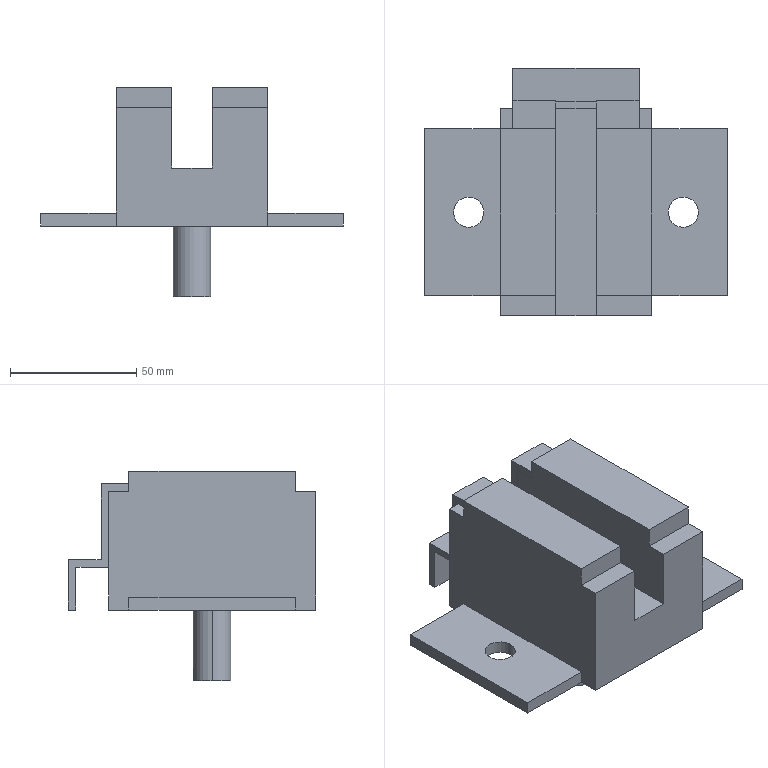Part | 2 solids | 51 faces | box 120 x 98 x 83 mm | volume 255571 mm3 | plane 45 | cylinder 6 | commonest cylinder face diameters 12 x4 15 x2
STEP:
#1=CARTESIAN_POINT('',(-48.5,0.,0.));
#2=VERTEX_POINT('',#1);
#3=CARTESIAN_POINT('',(-36.5,0.,0.));
#4=VERTEX_POINT('',#3);
#5=CARTESIAN_POINT('',(-42.5,0.,0.));
#6=DIRECTION('',(0.,0.,1.));
#7=DIRECTION('',(1.,0.,0.));
#8=AXIS2_PLACEMENT_3D('',#5,#6,#7);
#9=CIRCLE('',#8,6.);
#10=EDGE_CURVE('',#2,#4,#9,.T.);
#11=ORIENTED_EDGE('',*,*,#10,.F.);
#12=CARTESIAN_POINT('',(-48.5,0.,5.));
#13=VERTEX_POINT('',#12);
#14=CARTESIAN_POINT('',(-48.5,0.,-23.));
#15=DIRECTION('',(0.,0.,1.));
#16=VECTOR('',#15,1000.);
#17=LINE('',#14,#16);
#18=EDGE_CURVE('',#2,#13,#17,.T.);
#19=ORIENTED_EDGE('',*,*,#18,.T.);
#20=CARTESIAN_POINT('',(-36.5,0.,5.));
#21=VERTEX_POINT('',#20);
#22=CARTESIAN_POINT('',(-42.5,0.,5.));
#23=DIRECTION('',(0.,0.,1.));
#24=DIRECTION('',(1.,0.,0.));
#25=AXIS2_PLACEMENT_3D('',#22,#23,#24);
#26=CIRCLE('',#25,6.);
#27=EDGE_CURVE('',#13,#21,#26,.T.);
#28=ORIENTED_EDGE('',*,*,#27,.T.);
#29=CARTESIAN_POINT('',(-36.5,0.,-23.));
#30=DIRECTION('',(0.,0.,1.));
#31=VECTOR('',#30,1000.);
#32=LINE('',#29,#31);
#33=EDGE_CURVE('',#4,#21,#32,.T.);
#34=ORIENTED_EDGE('',*,*,#33,.F.);
#35=EDGE_LOOP('',(#11,#19,#28,#34));
#36=FACE_OUTER_BOUND('',#35,.T.);
#37=CARTESIAN_POINT('',(-42.5,0.,-23.));
#38=DIRECTION('',(0.,0.,1.));
#39=DIRECTION('',(1.,0.,0.));
#40=AXIS2_PLACEMENT_3D('',#37,#38,#39);
#41=CYLINDRICAL_SURFACE('',#40,6.);
#42=ADVANCED_FACE('',(#36),#41,.F.);
#43=CARTESIAN_POINT('',(36.5,0.,0.));
#44=VERTEX_POINT('',#43);
#45=CARTESIAN_POINT('',(48.5,0.,0.));
#46=VERTEX_POINT('',#45);
#47=CARTESIAN_POINT('',(42.5,0.,0.));
#48=DIRECTION('',(0.,0.,1.));
#49=DIRECTION('',(1.,0.,0.));
#50=AXIS2_PLACEMENT_3D('',#47,#48,#49);
#51=CIRCLE('',#50,6.);
#52=EDGE_CURVE('',#44,#46,#51,.T.);
#53=ORIENTED_EDGE('',*,*,#52,.F.);
#54=CARTESIAN_POINT('',(36.5,0.,5.));
#55=VERTEX_POINT('',#54);
#56=CARTESIAN_POINT('',(36.5,0.,-23.));
#57=DIRECTION('',(0.,0.,1.));
#58=VECTOR('',#57,1000.);
#59=LINE('',#56,#58);
#60=EDGE_CURVE('',#44,#55,#59,.T.);
#61=ORIENTED_EDGE('',*,*,#60,.T.);
#62=CARTESIAN_POINT('',(48.5,0.,5.));
#63=VERTEX_POINT('',#62);
#64=CARTESIAN_POINT('',(42.5,0.,5.));
#65=DIRECTION('',(0.,0.,1.));
#66=DIRECTION('',(-1.,0.,0.));
#67=AXIS2_PLACEMENT_3D('',#64,#65,#66);
#68=CIRCLE('',#67,6.);
#69=EDGE_CURVE('',#55,#63,#68,.T.);
#70=ORIENTED_EDGE('',*,*,#69,.T.);
#71=CARTESIAN_POINT('',(48.5,0.,-23.));
#72=DIRECTION('',(0.,0.,1.));
#73=VECTOR('',#72,1000.);
#74=LINE('',#71,#73);
#75=EDGE_CURVE('',#46,#63,#74,.T.);
#76=ORIENTED_EDGE('',*,*,#75,.F.);
#77=EDGE_LOOP('',(#53,#61,#70,#76));
#78=FACE_OUTER_BOUND('',#77,.T.);
#79=CARTESIAN_POINT('',(42.5,0.,-23.));
#80=DIRECTION('',(0.,0.,1.));
#81=DIRECTION('',(1.,0.,0.));
#82=AXIS2_PLACEMENT_3D('',#79,#80,#81);
#83=CYLINDRICAL_SURFACE('',#82,6.);
#84=ADVANCED_FACE('',(#78),#83,.F.);
#85=CARTESIAN_POINT('',(-7.5,0.,-28.));
#86=VERTEX_POINT('',#85);
#87=CARTESIAN_POINT('',(7.5,0.,-28.));
#88=VERTEX_POINT('',#87);
#89=CARTESIAN_POINT('',(0.,0.,-28.));
#90=DIRECTION('',(0.,0.,-1.));
#91=DIRECTION('',(-1.,0.,0.));
#92=AXIS2_PLACEMENT_3D('',#89,#90,#91);
#93=CIRCLE('',#92,7.5);
#94=EDGE_CURVE('',#86,#88,#93,.T.);
#95=ORIENTED_EDGE('',*,*,#94,.F.);
#96=CARTESIAN_POINT('',(-7.5,0.,0.));
#97=VERTEX_POINT('',#96);
#98=CARTESIAN_POINT('',(-7.5,0.,-28.));
#99=DIRECTION('',(0.,0.,1.));
#100=VECTOR('',#99,1000.);
#101=LINE('',#98,#100);
#102=EDGE_CURVE('',#86,#97,#101,.T.);
#103=ORIENTED_EDGE('',*,*,#102,.T.);
#104=CARTESIAN_POINT('',(7.5,0.,0.));
#105=VERTEX_POINT('',#104);
#106=CARTESIAN_POINT('',(0.,0.,0.));
#107=DIRECTION('',(0.,0.,-1.));
#108=DIRECTION('',(1.,0.,0.));
#109=AXIS2_PLACEMENT_3D('',#106,#107,#108);
#110=CIRCLE('',#109,7.5);
#111=EDGE_CURVE('',#97,#105,#110,.T.);
#112=ORIENTED_EDGE('',*,*,#111,.T.);
#113=CARTESIAN_POINT('',(7.5,0.,-28.));
#114=DIRECTION('',(0.,0.,1.));
#115=VECTOR('',#114,1000.);
#116=LINE('',#113,#115);
#117=EDGE_CURVE('',#88,#105,#116,.T.);
#118=ORIENTED_EDGE('',*,*,#117,.F.);
#119=EDGE_LOOP('',(#95,#103,#112,#118));
#120=FACE_OUTER_BOUND('',#119,.T.);
#121=CARTESIAN_POINT('',(0.,0.,-28.));
#122=DIRECTION('',(0.,0.,1.));
#123=DIRECTION('',(1.,0.,0.));
#124=AXIS2_PLACEMENT_3D('',#121,#122,#123);
#125=CYLINDRICAL_SURFACE('',#124,7.5);
#126=ADVANCED_FACE('',(#120),#125,.T.);
#127=CARTESIAN_POINT('',(30.,-33.,5.));
#128=VERTEX_POINT('',#127);
#129=CARTESIAN_POINT('',(60.,-33.,5.));
#130=VERTEX_POINT('',#129);
#131=CARTESIAN_POINT('',(-60.,-33.,5.));
#132=DIRECTION('',(1.,0.,0.));
#133=VECTOR('',#132,1000.);
#134=LINE('',#131,#133);
#135=EDGE_CURVE('',#128,#130,#134,.T.);
#136=ORIENTED_EDGE('',*,*,#135,.F.);
#137=CARTESIAN_POINT('',(30.,-33.,0.));
#138=VERTEX_POINT('',#137);
#139=CARTESIAN_POINT('',(30.,-33.,55.));
#140=DIRECTION('',(0.,0.,-1.));
#141=VECTOR('',#140,1000.);
#142=LINE('',#139,#141);
#143=EDGE_CURVE('',#128,#138,#142,.T.);
#144=ORIENTED_EDGE('',*,*,#143,.T.);
#145=CARTESIAN_POINT('',(60.,-33.,0.));
#146=VERTEX_POINT('',#145);
#147=CARTESIAN_POINT('',(-60.,-33.,0.));
#148=DIRECTION('',(1.,0.,0.));
#149=VECTOR('',#148,1000.);
#150=LINE('',#147,#149);
#151=EDGE_CURVE('',#138,#146,#150,.T.);
#152=ORIENTED_EDGE('',*,*,#151,.T.);
#153=CARTESIAN_POINT('',(60.,-33.,5.));
#154=DIRECTION('',(0.,0.,-1.));
#155=VECTOR('',#154,1000.);
#156=LINE('',#153,#155);
#157=EDGE_CURVE('',#130,#146,#156,.T.);
#158=ORIENTED_EDGE('',*,*,#157,.F.);
#159=EDGE_LOOP('',(#136,#144,#152,#158));
#160=FACE_OUTER_BOUND('',#159,.T.);
#161=CARTESIAN_POINT('',(-60.,-33.,5.));
#162=DIRECTION('',(0.,1.,0.));
#163=DIRECTION('',(0.,0.,1.));
#164=AXIS2_PLACEMENT_3D('',#161,#162,#163);
#165=PLANE('',#164);
#166=ADVANCED_FACE('',(#160),#165,.F.);
#167=CARTESIAN_POINT('',(-30.,33.,0.));
#168=VERTEX_POINT('',#167);
#169=CARTESIAN_POINT('',(-30.,33.,5.));
#170=VERTEX_POINT('',#169);
#171=CARTESIAN_POINT('',(-30.,33.,5.));
#172=DIRECTION('',(0.,0.,1.));
#173=VECTOR('',#172,1000.);
#174=LINE('',#171,#173);
#175=EDGE_CURVE('',#168,#170,#174,.T.);
#176=ORIENTED_EDGE('',*,*,#175,.F.);
#177=CARTESIAN_POINT('',(-60.,33.,0.));
#178=VERTEX_POINT('',#177);
#179=CARTESIAN_POINT('',(-60.,33.,0.));
#180=DIRECTION('',(-1.,0.,0.));
#181=VECTOR('',#180,1000.);
#182=LINE('',#179,#181);
#183=EDGE_CURVE('',#168,#178,#182,.T.);
#184=ORIENTED_EDGE('',*,*,#183,.T.);
#185=CARTESIAN_POINT('',(-60.,33.,5.));
#186=VERTEX_POINT('',#185);
#187=CARTESIAN_POINT('',(-60.,33.,5.));
#188=DIRECTION('',(0.,0.,-1.));
#189=VECTOR('',#188,1000.);
#190=LINE('',#187,#189);
#191=EDGE_CURVE('',#186,#178,#190,.T.);
#192=ORIENTED_EDGE('',*,*,#191,.F.);
#193=CARTESIAN_POINT('',(-60.,33.,5.));
#194=DIRECTION('',(-1.,0.,0.));
#195=VECTOR('',#194,1000.);
#196=LINE('',#193,#195);
#197=EDGE_CURVE('',#170,#186,#196,.T.);
#198=ORIENTED_EDGE('',*,*,#197,.F.);
#199=EDGE_LOOP('',(#176,#184,#192,#198));
#200=FACE_OUTER_BOUND('',#199,.T.);
#201=CARTESIAN_POINT('',(-60.,33.,5.));
#202=DIRECTION('',(0.,-1.,0.));
#203=DIRECTION('',(0.,0.,-1.));
#204=AXIS2_PLACEMENT_3D('',#201,#202,#203);
#205=PLANE('',#204);
#206=ADVANCED_FACE('',(#200),#205,.F.);
#207=CARTESIAN_POINT('',(30.,33.,5.));
#208=VERTEX_POINT('',#207);
#209=CARTESIAN_POINT('',(30.,33.,0.));
#210=VERTEX_POINT('',#209);
#211=CARTESIAN_POINT('',(30.,33.,5.));
#212=DIRECTION('',(0.,0.,-1.));
#213=VECTOR('',#212,1000.);
#214=LINE('',#211,#213);
#215=EDGE_CURVE('',#208,#210,#214,.T.);
#216=ORIENTED_EDGE('',*,*,#215,.F.);
#217=CARTESIAN_POINT('',(60.,33.,5.));
#218=VERTEX_POINT('',#217);
#219=CARTESIAN_POINT('',(-60.,33.,5.));
#220=DIRECTION('',(-1.,0.,0.));
#221=VECTOR('',#220,1000.);
#222=LINE('',#219,#221);
#223=EDGE_CURVE('',#218,#208,#222,.T.);
#224=ORIENTED_EDGE('',*,*,#223,.F.);
#225=CARTESIAN_POINT('',(60.,33.,0.));
#226=VERTEX_POINT('',#225);
#227=CARTESIAN_POINT('',(60.,33.,5.));
#228=DIRECTION('',(0.,0.,-1.));
#229=VECTOR('',#228,1000.);
#230=LINE('',#227,#229);
#231=EDGE_CURVE('',#218,#226,#230,.T.);
#232=ORIENTED_EDGE('',*,*,#231,.T.);
#233=CARTESIAN_POINT('',(-60.,33.,0.));
#234=DIRECTION('',(-1.,0.,0.));
#235=VECTOR('',#234,1000.);
#236=LINE('',#233,#235);
#237=EDGE_CURVE('',#226,#210,#236,.T.);
#238=ORIENTED_EDGE('',*,*,#237,.T.);
#239=EDGE_LOOP('',(#216,#224,#232,#238));
#240=FACE_OUTER_BOUND('',#239,.T.);
#241=CARTESIAN_POINT('',(-60.,33.,5.));
#242=DIRECTION('',(0.,-1.,0.));
#243=DIRECTION('',(0.,0.,-1.));
#244=AXIS2_PLACEMENT_3D('',#241,#242,#243);
#245=PLANE('',#244);
#246=ADVANCED_FACE('',(#240),#245,.F.);
#247=CARTESIAN_POINT('',(8.,33.,55.));
#248=VERTEX_POINT('',#247);
#249=CARTESIAN_POINT('',(30.,33.,55.));
#250=VERTEX_POINT('',#249);
#251=CARTESIAN_POINT('',(-60.,33.,55.));
#252=DIRECTION('',(1.,0.,0.));
#253=VECTOR('',#252,1000.);
#254=LINE('',#251,#253);
#255=EDGE_CURVE('',#248,#250,#254,.T.);
#256=ORIENTED_EDGE('',*,*,#255,.F.);
#257=CARTESIAN_POINT('',(8.,-33.,55.));
#258=VERTEX_POINT('',#257);
#259=CARTESIAN_POINT('',(8.,33.,55.));
#260=DIRECTION('',(0.,1.,0.));
#261=VECTOR('',#260,1000.);
#262=LINE('',#259,#261);
#263=EDGE_CURVE('',#258,#248,#262,.T.);
#264=ORIENTED_EDGE('',*,*,#263,.F.);
#265=CARTESIAN_POINT('',(30.,-33.,55.));
#266=VERTEX_POINT('',#265);
#267=CARTESIAN_POINT('',(-60.,-33.,55.));
#268=DIRECTION('',(1.,0.,0.));
#269=VECTOR('',#268,1000.);
#270=LINE('',#267,#269);
#271=EDGE_CURVE('',#258,#266,#270,.T.);
#272=ORIENTED_EDGE('',*,*,#271,.T.);
#273=CARTESIAN_POINT('',(30.,33.,55.));
#274=DIRECTION('',(0.,1.,0.));
#275=VECTOR('',#274,1000.);
#276=LINE('',#273,#275);
#277=EDGE_CURVE('',#266,#250,#276,.T.);
#278=ORIENTED_EDGE('',*,*,#277,.T.);
#279=EDGE_LOOP('',(#256,#264,#272,#278));
#280=FACE_OUTER_BOUND('',#279,.T.);
#281=CARTESIAN_POINT('',(0.,0.,55.));
#282=DIRECTION('',(0.,0.,1.));
#283=DIRECTION('',(1.,0.,0.));
#284=AXIS2_PLACEMENT_3D('',#281,#282,#283);
#285=PLANE('',#284);
#286=ADVANCED_FACE('',(#280),#285,.T.);
#287=CARTESIAN_POINT('',(42.5,0.,5.));
#288=DIRECTION('',(0.,0.,1.));
#289=DIRECTION('',(-1.,0.,0.));
#290=AXIS2_PLACEMENT_3D('',#287,#288,#289);
#291=CIRCLE('',#290,6.);
#292=EDGE_CURVE('',#63,#55,#291,.T.);
#293=ORIENTED_EDGE('',*,*,#292,.F.);
#294=ORIENTED_EDGE('',*,*,#69,.F.);
#295=EDGE_LOOP('',(#293,#294));
#296=FACE_BOUND('',#295,.T.);
#297=CARTESIAN_POINT('',(30.,33.,5.));
#298=DIRECTION('',(0.,1.,0.));
#299=VECTOR('',#298,1000.);
#300=LINE('',#297,#299);
#301=EDGE_CURVE('',#128,#208,#300,.T.);
#302=ORIENTED_EDGE('',*,*,#301,.F.);
#303=ORIENTED_EDGE('',*,*,#135,.T.);
#304=CARTESIAN_POINT('',(60.,33.,5.));
#305=DIRECTION('',(0.,1.,0.));
#306=VECTOR('',#305,1000.);
#307=LINE('',#304,#306);
#308=EDGE_CURVE('',#130,#218,#307,.T.);
#309=ORIENTED_EDGE('',*,*,#308,.T.);
#310=ORIENTED_EDGE('',*,*,#223,.T.);
#311=EDGE_LOOP('',(#302,#303,#309,#310));
#312=FACE_OUTER_BOUND('',#311,.T.);
#313=CARTESIAN_POINT('',(0.,0.,5.));
#314=DIRECTION('',(0.,0.,1.));
#315=DIRECTION('',(1.,0.,0.));
#316=AXIS2_PLACEMENT_3D('',#313,#314,#315);
#317=PLANE('',#316);
#318=ADVANCED_FACE('',(#296,#312),#317,.T.);
#319=CARTESIAN_POINT('',(60.,33.,0.));
#320=DIRECTION('',(0.,1.,0.));
#321=VECTOR('',#320,1000.);
#322=LINE('',#319,#321);
#323=EDGE_CURVE('',#146,#226,#322,.T.);
#324=ORIENTED_EDGE('',*,*,#323,.T.);
#325=ORIENTED_EDGE('',*,*,#231,.F.);
#326=ORIENTED_EDGE('',*,*,#308,.F.);
#327=ORIENTED_EDGE('',*,*,#157,.T.);
#328=EDGE_LOOP('',(#324,#325,#326,#327));
#329=FACE_OUTER_BOUND('',#328,.T.);
#330=CARTESIAN_POINT('',(60.,33.,5.));
#331=DIRECTION('',(-1.,0.,0.));
#332=DIRECTION('',(0.,-1.,0.));
#333=AXIS2_PLACEMENT_3D('',#330,#331,#332);
#334=PLANE('',#333);
#335=ADVANCED_FACE('',(#329),#334,.F.);
#336=CARTESIAN_POINT('',(-60.,-33.,0.));
#337=VERTEX_POINT('',#336);
#338=CARTESIAN_POINT('',(-60.,33.,0.));
#339=DIRECTION('',(0.,-1.,0.));
#340=VECTOR('',#339,1000.);
#341=LINE('',#338,#340);
#342=EDGE_CURVE('',#178,#337,#341,.T.);
#343=ORIENTED_EDGE('',*,*,#342,.T.);
#344=CARTESIAN_POINT('',(-60.,-33.,5.));
#345=VERTEX_POINT('',#344);
#346=CARTESIAN_POINT('',(-60.,-33.,5.));
#347=DIRECTION('',(0.,0.,-1.));
#348=VECTOR('',#347,1000.);
#349=LINE('',#346,#348);
#350=EDGE_CURVE('',#345,#337,#349,.T.);
#351=ORIENTED_EDGE('',*,*,#350,.F.);
#352=CARTESIAN_POINT('',(-60.,33.,5.));
#353=DIRECTION('',(0.,-1.,0.));
#354=VECTOR('',#353,1000.);
#355=LINE('',#352,#354);
#356=EDGE_CURVE('',#186,#345,#355,.T.);
#357=ORIENTED_EDGE('',*,*,#356,.F.);
#358=ORIENTED_EDGE('',*,*,#191,.T.);
#359=EDGE_LOOP('',(#343,#351,#357,#358));
#360=FACE_OUTER_BOUND('',#359,.T.);
#361=CARTESIAN_POINT('',(-60.,33.,5.));
#362=DIRECTION('',(1.,0.,0.));
#363=DIRECTION('',(0.,0.,-1.));
#364=AXIS2_PLACEMENT_3D('',#361,#362,#363);
#365=PLANE('',#364);
#366=ADVANCED_FACE('',(#360),#365,.F.);
#367=CARTESIAN_POINT('',(-30.,-33.,0.));
#368=VERTEX_POINT('',#367);
#369=CARTESIAN_POINT('',(-60.,-33.,0.));
#370=DIRECTION('',(1.,0.,0.));
#371=VECTOR('',#370,1000.);
#372=LINE('',#369,#371);
#373=EDGE_CURVE('',#337,#368,#372,.T.);
#374=ORIENTED_EDGE('',*,*,#373,.T.);
#375=CARTESIAN_POINT('',(-30.,-33.,5.));
#376=VERTEX_POINT('',#375);
#377=CARTESIAN_POINT('',(-30.,-33.,5.));
#378=DIRECTION('',(0.,0.,1.));
#379=VECTOR('',#378,1000.);
#380=LINE('',#377,#379);
#381=EDGE_CURVE('',#368,#376,#380,.T.);
#382=ORIENTED_EDGE('',*,*,#381,.T.);
#383=CARTESIAN_POINT('',(-60.,-33.,5.));
#384=DIRECTION('',(1.,0.,0.));
#385=VECTOR('',#384,1000.);
#386=LINE('',#383,#385);
#387=EDGE_CURVE('',#345,#376,#386,.T.);
#388=ORIENTED_EDGE('',*,*,#387,.F.);
#389=ORIENTED_EDGE('',*,*,#350,.T.);
#390=EDGE_LOOP('',(#374,#382,#388,#389));
#391=FACE_OUTER_BOUND('',#390,.T.);
#392=CARTESIAN_POINT('',(-60.,-33.,5.));
#393=DIRECTION('',(0.,1.,0.));
#394=DIRECTION('',(0.,0.,1.));
#395=AXIS2_PLACEMENT_3D('',#392,#393,#394);
#396=PLANE('',#395);
#397=ADVANCED_FACE('',(#391),#396,.F.);
#398=CARTESIAN_POINT('',(-42.5,0.,5.));
#399=DIRECTION('',(0.,0.,1.));
#400=DIRECTION('',(1.,0.,0.));
#401=AXIS2_PLACEMENT_3D('',#398,#399,#400);
#402=CIRCLE('',#401,6.);
#403=EDGE_CURVE('',#21,#13,#402,.T.);
#404=ORIENTED_EDGE('',*,*,#403,.F.);
#405=ORIENTED_EDGE('',*,*,#27,.F.);
#406=EDGE_LOOP('',(#404,#405));
#407=FACE_BOUND('',#406,.T.);
#408=CARTESIAN_POINT('',(-30.,33.,5.));
#409=DIRECTION('',(0.,-1.,0.));
#410=VECTOR('',#409,1000.);
#411=LINE('',#408,#410);
#412=EDGE_CURVE('',#170,#376,#411,.T.);
#413=ORIENTED_EDGE('',*,*,#412,.F.);
#414=ORIENTED_EDGE('',*,*,#197,.T.);
#415=ORIENTED_EDGE('',*,*,#356,.T.);
#416=ORIENTED_EDGE('',*,*,#387,.T.);
#417=EDGE_LOOP('',(#413,#414,#415,#416));
#418=FACE_OUTER_BOUND('',#417,.T.);
#419=CARTESIAN_POINT('',(0.,0.,5.));
#420=DIRECTION('',(0.,0.,1.));
#421=DIRECTION('',(1.,0.,0.));
#422=AXIS2_PLACEMENT_3D('',#419,#420,#421);
#423=PLANE('',#422);
#424=ADVANCED_FACE('',(#407,#418),#423,.T.);
#425=CARTESIAN_POINT('',(-42.5,0.,0.));
#426=DIRECTION('',(0.,0.,1.));
#427=DIRECTION('',(1.,0.,0.));
#428=AXIS2_PLACEMENT_3D('',#425,#426,#427);
#429=CIRCLE('',#428,6.);
#430=EDGE_CURVE('',#4,#2,#429,.T.);
#431=ORIENTED_EDGE('',*,*,#430,.T.);
#432=ORIENTED_EDGE('',*,*,#10,.T.);
#433=EDGE_LOOP('',(#431,#432));
#434=FACE_BOUND('',#433,.T.);
#435=CARTESIAN_POINT('',(42.5,0.,0.));
#436=DIRECTION('',(0.,0.,1.));
#437=DIRECTION('',(1.,0.,0.));
#438=AXIS2_PLACEMENT_3D('',#435,#436,#437);
#439=CIRCLE('',#438,6.);
#440=EDGE_CURVE('',#46,#44,#439,.T.);
#441=ORIENTED_EDGE('',*,*,#440,.T.);
#442=ORIENTED_EDGE('',*,*,#52,.T.);
#443=EDGE_LOOP('',(#441,#442));
#444=FACE_BOUND('',#443,.T.);
#445=CARTESIAN_POINT('',(0.,0.,0.));
#446=DIRECTION('',(0.,0.,-1.));
#447=DIRECTION('',(1.,0.,0.));
#448=AXIS2_PLACEMENT_3D('',#445,#446,#447);
#449=CIRCLE('',#448,7.5);
#450=EDGE_CURVE('',#105,#97,#449,.T.);
#451=ORIENTED_EDGE('',*,*,#450,.F.);
#452=ORIENTED_EDGE('',*,*,#111,.F.);
#453=EDGE_LOOP('',(#451,#452));
#454=FACE_BOUND('',#453,.T.);
#455=ORIENTED_EDGE('',*,*,#323,.F.);
#456=ORIENTED_EDGE('',*,*,#151,.F.);
#457=CARTESIAN_POINT('',(30.,-41.,0.));
#458=VERTEX_POINT('',#457);
#459=CARTESIAN_POINT('',(30.,-41.,0.));
#460=DIRECTION('',(0.,1.,0.));
#461=VECTOR('',#460,1000.);
#462=LINE('',#459,#461);
#463=EDGE_CURVE('',#458,#138,#462,.T.);
#464=ORIENTED_EDGE('',*,*,#463,.F.);
#465=CARTESIAN_POINT('',(-30.,-41.,0.));
#466=VERTEX_POINT('',#465);
#467=CARTESIAN_POINT('',(30.,-41.,0.));
#468=DIRECTION('',(-1.,0.,0.));
#469=VECTOR('',#468,1000.);
#470=LINE('',#467,#469);
#471=EDGE_CURVE('',#458,#466,#470,.T.);
#472=ORIENTED_EDGE('',*,*,#471,.T.);
#473=CARTESIAN_POINT('',(-30.,-41.,0.));
#474=DIRECTION('',(0.,1.,0.));
#475=VECTOR('',#474,1000.);
#476=LINE('',#473,#475);
#477=EDGE_CURVE('',#466,#368,#476,.T.);
#478=ORIENTED_EDGE('',*,*,#477,.T.);
#479=ORIENTED_EDGE('',*,*,#373,.F.);
#480=ORIENTED_EDGE('',*,*,#342,.F.);
#481=ORIENTED_EDGE('',*,*,#183,.F.);
#482=CARTESIAN_POINT('',(-30.,41.,0.));
#483=VERTEX_POINT('',#482);
#484=CARTESIAN_POINT('',(-30.,41.,0.));
#485=DIRECTION('',(0.,-1.,0.));
#486=VECTOR('',#485,1000.);
#487=LINE('',#484,#486);
#488=EDGE_CURVE('',#483,#168,#487,.T.);
#489=ORIENTED_EDGE('',*,*,#488,.F.);
#490=CARTESIAN_POINT('',(30.,41.,0.));
#491=VERTEX_POINT('',#490);
#492=CARTESIAN_POINT('',(30.,41.,0.));
#493=DIRECTION('',(-1.,0.,0.));
#494=VECTOR('',#493,1000.);
#495=LINE('',#492,#494);
#496=EDGE_CURVE('',#491,#483,#495,.T.);
#497=ORIENTED_EDGE('',*,*,#496,.F.);
#498=CARTESIAN_POINT('',(30.,41.,0.));
#499=DIRECTION('',(0.,-1.,0.));
#500=VECTOR('',#499,1000.);
#501=LINE('',#498,#500);
#502=EDGE_CURVE('',#491,#210,#501,.T.);
#503=ORIENTED_EDGE('',*,*,#502,.T.);
#504=ORIENTED_EDGE('',*,*,#237,.F.);
#505=EDGE_LOOP('',(#455,#456,#464,#472,#478,#479,#480,#481,#489,#497,#503,#504));
#506=FACE_OUTER_BOUND('',#505,.T.);
#507=CARTESIAN_POINT('',(0.,0.,0.));
#508=DIRECTION('',(0.,0.,1.));
#509=DIRECTION('',(1.,0.,0.));
#510=AXIS2_PLACEMENT_3D('',#507,#508,#509);
#511=PLANE('',#510);
#512=ADVANCED_FACE('',(#434,#444,#454,#506),#511,.F.);
#513=CARTESIAN_POINT('',(30.,41.,47.));
#514=VERTEX_POINT('',#513);
#515=CARTESIAN_POINT('',(30.,41.,55.));
#516=DIRECTION('',(0.,0.,-1.));
#517=VECTOR('',#516,1000.);
#518=LINE('',#515,#517);
#519=EDGE_CURVE('',#514,#491,#518,.T.);
#520=ORIENTED_EDGE('',*,*,#519,.F.);
#521=CARTESIAN_POINT('',(30.,33.,47.));
#522=VERTEX_POINT('',#521);
#523=CARTESIAN_POINT('',(30.,33.,47.));
#524=DIRECTION('',(0.,-1.,0.));
#525=VECTOR('',#524,1000.);
#526=LINE('',#523,#525);
#527=EDGE_CURVE('',#514,#522,#526,.T.);
#528=ORIENTED_EDGE('',*,*,#527,.T.);
#529=CARTESIAN_POINT('',(30.,33.,55.));
#530=DIRECTION('',(0.,0.,1.));
#531=VECTOR('',#530,1000.);
#532=LINE('',#529,#531);
#533=EDGE_CURVE('',#522,#250,#532,.T.);
#534=ORIENTED_EDGE('',*,*,#533,.T.);
#535=ORIENTED_EDGE('',*,*,#277,.F.);
#536=CARTESIAN_POINT('',(30.,-33.,47.));
#537=VERTEX_POINT('',#536);
#538=CARTESIAN_POINT('',(30.,-33.,55.));
#539=DIRECTION('',(0.,0.,-1.));
#540=VECTOR('',#539,1000.);
#541=LINE('',#538,#540);
#542=EDGE_CURVE('',#266,#537,#541,.T.);
#543=ORIENTED_EDGE('',*,*,#542,.T.);
#544=CARTESIAN_POINT('',(30.,-41.,47.));
#545=VERTEX_POINT('',#544);
#546=CARTESIAN_POINT('',(30.,33.,47.));
#547=DIRECTION('',(0.,-1.,0.));
#548=VECTOR('',#547,1000.);
#549=LINE('',#546,#548);
#550=EDGE_CURVE('',#537,#545,#549,.T.);
#551=ORIENTED_EDGE('',*,*,#550,.T.);
#552=CARTESIAN_POINT('',(30.,-41.,5.));
#553=DIRECTION('',(0.,0.,-1.));
#554=VECTOR('',#553,1000.);
#555=LINE('',#552,#554);
#556=EDGE_CURVE('',#545,#458,#555,.T.);
#557=ORIENTED_EDGE('',*,*,#556,.T.);
#558=ORIENTED_EDGE('',*,*,#463,.T.);
#559=ORIENTED_EDGE('',*,*,#143,.F.);
#560=ORIENTED_EDGE('',*,*,#301,.T.);
#561=ORIENTED_EDGE('',*,*,#215,.T.);
#562=ORIENTED_EDGE('',*,*,#502,.F.);
#563=EDGE_LOOP('',(#520,#528,#534,#535,#543,#551,#557,#558,#559,#560,#561,#562));
#564=FACE_OUTER_BOUND('',#563,.T.);
#565=CARTESIAN_POINT('',(30.,33.,55.));
#566=DIRECTION('',(-1.,0.,0.));
#567=DIRECTION('',(0.,0.,1.));
#568=AXIS2_PLACEMENT_3D('',#565,#566,#567);
#569=PLANE('',#568);
#570=ADVANCED_FACE('',(#564),#569,.F.);
#571=CARTESIAN_POINT('',(-30.,33.,55.));
#572=VERTEX_POINT('',#571);
#573=CARTESIAN_POINT('',(-30.,33.,47.));
#574=VERTEX_POINT('',#573);
#575=CARTESIAN_POINT('',(-30.,33.,55.));
#576=DIRECTION('',(0.,0.,-1.));
#577=VECTOR('',#576,1000.);
#578=LINE('',#575,#577);
#579=EDGE_CURVE('',#572,#574,#578,.T.);
#580=ORIENTED_EDGE('',*,*,#579,.T.);
#581=CARTESIAN_POINT('',(-30.,41.,47.));
#582=VERTEX_POINT('',#581);
#583=CARTESIAN_POINT('',(-30.,33.,47.));
#584=DIRECTION('',(0.,1.,0.));
#585=VECTOR('',#584,1000.);
#586=LINE('',#583,#585);
#587=EDGE_CURVE('',#574,#582,#586,.T.);
#588=ORIENTED_EDGE('',*,*,#587,.T.);
#589=CARTESIAN_POINT('',(-30.,41.,5.));
#590=DIRECTION('',(0.,0.,1.));
#591=VECTOR('',#590,1000.);
#592=LINE('',#589,#591);
#593=EDGE_CURVE('',#483,#582,#592,.T.);
#594=ORIENTED_EDGE('',*,*,#593,.F.);
#595=ORIENTED_EDGE('',*,*,#488,.T.);
#596=ORIENTED_EDGE('',*,*,#175,.T.);
#597=ORIENTED_EDGE('',*,*,#412,.T.);
#598=ORIENTED_EDGE('',*,*,#381,.F.);
#599=ORIENTED_EDGE('',*,*,#477,.F.);
#600=CARTESIAN_POINT('',(-30.,-41.,47.));
#601=VERTEX_POINT('',#600);
#602=CARTESIAN_POINT('',(-30.,-41.,5.));
#603=DIRECTION('',(0.,0.,1.));
#604=VECTOR('',#603,1000.);
#605=LINE('',#602,#604);
#606=EDGE_CURVE('',#466,#601,#605,.T.);
#607=ORIENTED_EDGE('',*,*,#606,.T.);
#608=CARTESIAN_POINT('',(-30.,-33.,47.));
#609=VERTEX_POINT('',#608);
#610=CARTESIAN_POINT('',(-30.,33.,47.));
#611=DIRECTION('',(0.,1.,0.));
#612=VECTOR('',#611,1000.);
#613=LINE('',#610,#612);
#614=EDGE_CURVE('',#601,#609,#613,.T.);
#615=ORIENTED_EDGE('',*,*,#614,.T.);
#616=CARTESIAN_POINT('',(-30.,-33.,55.));
#617=VERTEX_POINT('',#616);
#618=CARTESIAN_POINT('',(-30.,-33.,55.));
#619=DIRECTION('',(0.,0.,1.));
#620=VECTOR('',#619,1000.);
#621=LINE('',#618,#620);
#622=EDGE_CURVE('',#609,#617,#621,.T.);
#623=ORIENTED_EDGE('',*,*,#622,.T.);
#624=CARTESIAN_POINT('',(-30.,33.,55.));
#625=DIRECTION('',(0.,-1.,0.));
#626=VECTOR('',#625,1000.);
#627=LINE('',#624,#626);
#628=EDGE_CURVE('',#572,#617,#627,.T.);
#629=ORIENTED_EDGE('',*,*,#628,.F.);
#630=EDGE_LOOP('',(#580,#588,#594,#595,#596,#597,#598,#599,#607,#615,#623,#629));
#631=FACE_OUTER_BOUND('',#630,.T.);
#632=CARTESIAN_POINT('',(-30.,33.,55.));
#633=DIRECTION('',(1.,0.,0.));
#634=DIRECTION('',(0.,0.,-1.));
#635=AXIS2_PLACEMENT_3D('',#632,#633,#634);
#636=PLANE('',#635);
#637=ADVANCED_FACE('',(#631),#636,.F.);
#638=CARTESIAN_POINT('',(-8.,33.,55.));
#639=VERTEX_POINT('',#638);
#640=CARTESIAN_POINT('',(-60.,33.,55.));
#641=DIRECTION('',(1.,0.,0.));
#642=VECTOR('',#641,1000.);
#643=LINE('',#640,#642);
#644=EDGE_CURVE('',#572,#639,#643,.T.);
#645=ORIENTED_EDGE('',*,*,#644,.F.);
#646=ORIENTED_EDGE('',*,*,#628,.T.);
#647=CARTESIAN_POINT('',(-8.,-33.,55.));
#648=VERTEX_POINT('',#647);
#649=CARTESIAN_POINT('',(-60.,-33.,55.));
#650=DIRECTION('',(1.,0.,0.));
#651=VECTOR('',#650,1000.);
#652=LINE('',#649,#651);
#653=EDGE_CURVE('',#617,#648,#652,.T.);
#654=ORIENTED_EDGE('',*,*,#653,.T.);
#655=CARTESIAN_POINT('',(-8.,33.,55.));
#656=DIRECTION('',(0.,-1.,0.));
#657=VECTOR('',#656,1000.);
#658=LINE('',#655,#657);
#659=EDGE_CURVE('',#639,#648,#658,.T.);
#660=ORIENTED_EDGE('',*,*,#659,.F.);
#661=EDGE_LOOP('',(#645,#646,#654,#660));
#662=FACE_OUTER_BOUND('',#661,.T.);
#663=CARTESIAN_POINT('',(0.,0.,55.));
#664=DIRECTION('',(0.,0.,1.));
#665=DIRECTION('',(1.,0.,0.));
#666=AXIS2_PLACEMENT_3D('',#663,#664,#665);
#667=PLANE('',#666);
#668=ADVANCED_FACE('',(#662),#667,.T.);
#669=CARTESIAN_POINT('',(8.,33.,47.));
#670=VERTEX_POINT('',#669);
#671=CARTESIAN_POINT('',(8.,33.,23.));
#672=DIRECTION('',(0.,0.,-1.));
#673=VECTOR('',#672,1000.);
#674=LINE('',#671,#673);
#675=EDGE_CURVE('',#248,#670,#674,.T.);
#676=ORIENTED_EDGE('',*,*,#675,.T.);
#677=CARTESIAN_POINT('',(8.,41.,47.));
#678=VERTEX_POINT('',#677);
#679=CARTESIAN_POINT('',(8.,33.,47.));
#680=DIRECTION('',(0.,1.,0.));
#681=VECTOR('',#680,1000.);
#682=LINE('',#679,#681);
#683=EDGE_CURVE('',#670,#678,#682,.T.);
#684=ORIENTED_EDGE('',*,*,#683,.T.);
#685=CARTESIAN_POINT('',(8.,41.,23.));
#686=VERTEX_POINT('',#685);
#687=CARTESIAN_POINT('',(8.,41.,23.));
#688=DIRECTION('',(0.,0.,1.));
#689=VECTOR('',#688,1000.);
#690=LINE('',#687,#689);
#691=EDGE_CURVE('',#686,#678,#690,.T.);
#692=ORIENTED_EDGE('',*,*,#691,.F.);
#693=CARTESIAN_POINT('',(8.,-41.,23.));
#694=VERTEX_POINT('',#693);
#695=CARTESIAN_POINT('',(8.,33.,23.));
#696=DIRECTION('',(0.,1.,0.));
#697=VECTOR('',#696,1000.);
#698=LINE('',#695,#697);
#699=EDGE_CURVE('',#694,#686,#698,.T.);
#700=ORIENTED_EDGE('',*,*,#699,.F.);
#701=CARTESIAN_POINT('',(8.,-41.,47.));
#702=VERTEX_POINT('',#701);
#703=CARTESIAN_POINT('',(8.,-41.,23.));
#704=DIRECTION('',(0.,0.,1.));
#705=VECTOR('',#704,1000.);
#706=LINE('',#703,#705);
#707=EDGE_CURVE('',#694,#702,#706,.T.);
#708=ORIENTED_EDGE('',*,*,#707,.T.);
#709=CARTESIAN_POINT('',(8.,-33.,47.));
#710=VERTEX_POINT('',#709);
#711=CARTESIAN_POINT('',(8.,33.,47.));
#712=DIRECTION('',(0.,1.,0.));
#713=VECTOR('',#712,1000.);
#714=LINE('',#711,#713);
#715=EDGE_CURVE('',#702,#710,#714,.T.);
#716=ORIENTED_EDGE('',*,*,#715,.T.);
#717=CARTESIAN_POINT('',(8.,-33.,23.));
#718=DIRECTION('',(0.,0.,1.));
#719=VECTOR('',#718,1000.);
#720=LINE('',#717,#719);
#721=EDGE_CURVE('',#710,#258,#720,.T.);
#722=ORIENTED_EDGE('',*,*,#721,.T.);
#723=ORIENTED_EDGE('',*,*,#263,.T.);
#724=EDGE_LOOP('',(#676,#684,#692,#700,#708,#716,#722,#723));
#725=FACE_OUTER_BOUND('',#724,.T.);
#726=CARTESIAN_POINT('',(8.,33.,23.));
#727=DIRECTION('',(1.,0.,0.));
#728=DIRECTION('',(0.,0.,-1.));
#729=AXIS2_PLACEMENT_3D('',#726,#727,#728);
#730=PLANE('',#729);
#731=ADVANCED_FACE('',(#725),#730,.F.);
#732=CARTESIAN_POINT('',(-8.,-33.,47.));
#733=VERTEX_POINT('',#732);
#734=CARTESIAN_POINT('',(-8.,-33.,23.));
#735=DIRECTION('',(0.,0.,-1.));
#736=VECTOR('',#735,1000.);
#737=LINE('',#734,#736);
#738=EDGE_CURVE('',#648,#733,#737,.T.);
#739=ORIENTED_EDGE('',*,*,#738,.T.);
#740=CARTESIAN_POINT('',(-8.,-41.,47.));
#741=VERTEX_POINT('',#740);
#742=CARTESIAN_POINT('',(-8.,33.,47.));
#743=DIRECTION('',(0.,-1.,0.));
#744=VECTOR('',#743,1000.);
#745=LINE('',#742,#744);
#746=EDGE_CURVE('',#733,#741,#745,.T.);
#747=ORIENTED_EDGE('',*,*,#746,.T.);
#748=CARTESIAN_POINT('',(-8.,-41.,23.));
#749=VERTEX_POINT('',#748);
#750=CARTESIAN_POINT('',(-8.,-41.,55.));
#751=DIRECTION('',(0.,0.,-1.));
#752=VECTOR('',#751,1000.);
#753=LINE('',#750,#752);
#754=EDGE_CURVE('',#741,#749,#753,.T.);
#755=ORIENTED_EDGE('',*,*,#754,.T.);
#756=CARTESIAN_POINT('',(-8.,41.,23.));
#757=VERTEX_POINT('',#756);
#758=CARTESIAN_POINT('',(-8.,33.,23.));
#759=DIRECTION('',(0.,-1.,0.));
#760=VECTOR('',#759,1000.);
#761=LINE('',#758,#760);
#762=EDGE_CURVE('',#757,#749,#761,.T.);
#763=ORIENTED_EDGE('',*,*,#762,.F.);
#764=CARTESIAN_POINT('',(-8.,41.,47.));
#765=VERTEX_POINT('',#764);
#766=CARTESIAN_POINT('',(-8.,41.,55.));
#767=DIRECTION('',(0.,0.,-1.));
#768=VECTOR('',#767,1000.);
#769=LINE('',#766,#768);
#770=EDGE_CURVE('',#765,#757,#769,.T.);
#771=ORIENTED_EDGE('',*,*,#770,.F.);
#772=CARTESIAN_POINT('',(-8.,33.,47.));
#773=VERTEX_POINT('',#772);
#774=CARTESIAN_POINT('',(-8.,33.,47.));
#775=DIRECTION('',(0.,-1.,0.));
#776=VECTOR('',#775,1000.);
#777=LINE('',#774,#776);
#778=EDGE_CURVE('',#765,#773,#777,.T.);
#779=ORIENTED_EDGE('',*,*,#778,.T.);
#780=CARTESIAN_POINT('',(-8.,33.,23.));
#781=DIRECTION('',(0.,0.,1.));
#782=VECTOR('',#781,1000.);
#783=LINE('',#780,#782);
#784=EDGE_CURVE('',#773,#639,#783,.T.);
#785=ORIENTED_EDGE('',*,*,#784,.T.);
#786=ORIENTED_EDGE('',*,*,#659,.T.);
#787=EDGE_LOOP('',(#739,#747,#755,#763,#771,#779,#785,#786));
#788=FACE_OUTER_BOUND('',#787,.T.);
#789=CARTESIAN_POINT('',(-8.,33.,23.));
#790=DIRECTION('',(-1.,0.,0.));
#791=DIRECTION('',(0.,0.,1.));
#792=AXIS2_PLACEMENT_3D('',#789,#790,#791);
#793=PLANE('',#792);
#794=ADVANCED_FACE('',(#788),#793,.F.);
#795=ORIENTED_EDGE('',*,*,#699,.T.);
#796=CARTESIAN_POINT('',(-8.,41.,23.));
#797=DIRECTION('',(1.,0.,0.));
#798=VECTOR('',#797,1000.);
#799=LINE('',#796,#798);
#800=EDGE_CURVE('',#757,#686,#799,.T.);
#801=ORIENTED_EDGE('',*,*,#800,.F.);
#802=ORIENTED_EDGE('',*,*,#762,.T.);
#803=CARTESIAN_POINT('',(-8.,-41.,23.));
#804=DIRECTION('',(1.,0.,0.));
#805=VECTOR('',#804,1000.);
#806=LINE('',#803,#805);
#807=EDGE_CURVE('',#749,#694,#806,.T.);
#808=ORIENTED_EDGE('',*,*,#807,.T.);
#809=EDGE_LOOP('',(#795,#801,#802,#808));
#810=FACE_OUTER_BOUND('',#809,.T.);
#811=CARTESIAN_POINT('',(0.,0.,23.));
#812=DIRECTION('',(0.,0.,1.));
#813=DIRECTION('',(1.,0.,0.));
#814=AXIS2_PLACEMENT_3D('',#811,#812,#813);
#815=PLANE('',#814);
#816=ADVANCED_FACE('',(#810),#815,.T.);
#817=ORIENTED_EDGE('',*,*,#102,.F.);
#818=CARTESIAN_POINT('',(0.,0.,-28.));
#819=DIRECTION('',(0.,0.,-1.));
#820=DIRECTION('',(-1.,0.,0.));
#821=AXIS2_PLACEMENT_3D('',#818,#819,#820);
#822=CIRCLE('',#821,7.5);
#823=EDGE_CURVE('',#88,#86,#822,.T.);
#824=ORIENTED_EDGE('',*,*,#823,.F.);
#825=ORIENTED_EDGE('',*,*,#117,.T.);
#826=ORIENTED_EDGE('',*,*,#450,.T.);
#827=EDGE_LOOP('',(#817,#824,#825,#826));
#828=FACE_OUTER_BOUND('',#827,.T.);
#829=CARTESIAN_POINT('',(0.,0.,-28.));
#830=DIRECTION('',(0.,0.,1.));
#831=DIRECTION('',(1.,0.,0.));
#832=AXIS2_PLACEMENT_3D('',#829,#830,#831);
#833=CYLINDRICAL_SURFACE('',#832,7.5);
#834=ADVANCED_FACE('',(#828),#833,.T.);
#835=ORIENTED_EDGE('',*,*,#823,.T.);
#836=ORIENTED_EDGE('',*,*,#94,.T.);
#837=EDGE_LOOP('',(#835,#836));
#838=FACE_OUTER_BOUND('',#837,.T.);
#839=CARTESIAN_POINT('',(0.,0.,-28.));
#840=DIRECTION('',(0.,0.,-1.));
#841=DIRECTION('',(-1.,0.,0.));
#842=AXIS2_PLACEMENT_3D('',#839,#840,#841);
#843=PLANE('',#842);
#844=ADVANCED_FACE('',(#838),#843,.T.);
#845=ORIENTED_EDGE('',*,*,#60,.F.);
#846=ORIENTED_EDGE('',*,*,#440,.F.);
#847=ORIENTED_EDGE('',*,*,#75,.T.);
#848=ORIENTED_EDGE('',*,*,#292,.T.);
#849=EDGE_LOOP('',(#845,#846,#847,#848));
#850=FACE_OUTER_BOUND('',#849,.T.);
#851=CARTESIAN_POINT('',(42.5,0.,-23.));
#852=DIRECTION('',(0.,0.,1.));
#853=DIRECTION('',(1.,0.,0.));
#854=AXIS2_PLACEMENT_3D('',#851,#852,#853);
#855=CYLINDRICAL_SURFACE('',#854,6.);
#856=ADVANCED_FACE('',(#850),#855,.F.);
#857=ORIENTED_EDGE('',*,*,#18,.F.);
#858=ORIENTED_EDGE('',*,*,#430,.F.);
#859=ORIENTED_EDGE('',*,*,#33,.T.);
#860=ORIENTED_EDGE('',*,*,#403,.T.);
#861=EDGE_LOOP('',(#857,#858,#859,#860));
#862=FACE_OUTER_BOUND('',#861,.T.);
#863=CARTESIAN_POINT('',(-42.5,0.,-23.));
#864=DIRECTION('',(0.,0.,1.));
#865=DIRECTION('',(1.,0.,0.));
#866=AXIS2_PLACEMENT_3D('',#863,#864,#865);
#867=CYLINDRICAL_SURFACE('',#866,6.);
#868=ADVANCED_FACE('',(#862),#867,.F.);
#869=ORIENTED_EDGE('',*,*,#593,.T.);
#870=CARTESIAN_POINT('',(0.,41.,47.));
#871=DIRECTION('',(1.,0.,0.));
#872=VECTOR('',#871,1000.);
#873=LINE('',#870,#872);
#874=EDGE_CURVE('',#582,#765,#873,.T.);
#875=ORIENTED_EDGE('',*,*,#874,.T.);
#876=ORIENTED_EDGE('',*,*,#770,.T.);
#877=ORIENTED_EDGE('',*,*,#800,.T.);
#878=ORIENTED_EDGE('',*,*,#691,.T.);
#879=CARTESIAN_POINT('',(0.,41.,47.));
#880=DIRECTION('',(1.,0.,0.));
#881=VECTOR('',#880,1000.);
#882=LINE('',#879,#881);
#883=EDGE_CURVE('',#678,#514,#882,.T.);
#884=ORIENTED_EDGE('',*,*,#883,.T.);
#885=ORIENTED_EDGE('',*,*,#519,.T.);
#886=ORIENTED_EDGE('',*,*,#496,.T.);
#887=EDGE_LOOP('',(#869,#875,#876,#877,#878,#884,#885,#886));
#888=FACE_OUTER_BOUND('',#887,.T.);
#889=CARTESIAN_POINT('',(0.,41.,0.));
#890=DIRECTION('',(0.,-1.,0.));
#891=DIRECTION('',(0.,0.,-1.));
#892=AXIS2_PLACEMENT_3D('',#889,#890,#891);
#893=PLANE('',#892);
#894=ADVANCED_FACE('',(#888),#893,.F.);
#895=ORIENTED_EDGE('',*,*,#556,.F.);
#896=CARTESIAN_POINT('',(0.,-41.,47.));
#897=DIRECTION('',(-1.,0.,0.));
#898=VECTOR('',#897,1000.);
#899=LINE('',#896,#898);
#900=EDGE_CURVE('',#545,#702,#899,.T.);
#901=ORIENTED_EDGE('',*,*,#900,.T.);
#902=ORIENTED_EDGE('',*,*,#707,.F.);
#903=ORIENTED_EDGE('',*,*,#807,.F.);
#904=ORIENTED_EDGE('',*,*,#754,.F.);
#905=CARTESIAN_POINT('',(0.,-41.,47.));
#906=DIRECTION('',(-1.,0.,0.));
#907=VECTOR('',#906,1000.);
#908=LINE('',#905,#907);
#909=EDGE_CURVE('',#741,#601,#908,.T.);
#910=ORIENTED_EDGE('',*,*,#909,.T.);
#911=ORIENTED_EDGE('',*,*,#606,.F.);
#912=ORIENTED_EDGE('',*,*,#471,.F.);
#913=EDGE_LOOP('',(#895,#901,#902,#903,#904,#910,#911,#912));
#914=FACE_OUTER_BOUND('',#913,.T.);
#915=CARTESIAN_POINT('',(0.,-41.,0.));
#916=DIRECTION('',(0.,1.,0.));
#917=DIRECTION('',(0.,0.,-1.));
#918=AXIS2_PLACEMENT_3D('',#915,#916,#917);
#919=PLANE('',#918);
#920=ADVANCED_FACE('',(#914),#919,.F.);
#921=ORIENTED_EDGE('',*,*,#909,.F.);
#922=ORIENTED_EDGE('',*,*,#746,.F.);
#923=CARTESIAN_POINT('',(-60.,-33.,47.));
#924=DIRECTION('',(1.,0.,0.));
#925=VECTOR('',#924,1000.);
#926=LINE('',#923,#925);
#927=EDGE_CURVE('',#609,#733,#926,.T.);
#928=ORIENTED_EDGE('',*,*,#927,.F.);
#929=ORIENTED_EDGE('',*,*,#614,.F.);
#930=EDGE_LOOP('',(#921,#922,#928,#929));
#931=FACE_OUTER_BOUND('',#930,.T.);
#932=CARTESIAN_POINT('',(-60.,-33.,47.));
#933=DIRECTION('',(0.,0.,-1.));
#934=DIRECTION('',(-1.,0.,0.));
#935=AXIS2_PLACEMENT_3D('',#932,#933,#934);
#936=PLANE('',#935);
#937=ADVANCED_FACE('',(#931),#936,.F.);
#938=ORIENTED_EDGE('',*,*,#927,.T.);
#939=ORIENTED_EDGE('',*,*,#738,.F.);
#940=ORIENTED_EDGE('',*,*,#653,.F.);
#941=ORIENTED_EDGE('',*,*,#622,.F.);
#942=EDGE_LOOP('',(#938,#939,#940,#941));
#943=FACE_OUTER_BOUND('',#942,.T.);
#944=CARTESIAN_POINT('',(-60.,-33.,55.));
#945=DIRECTION('',(0.,1.,0.));
#946=DIRECTION('',(0.,0.,1.));
#947=AXIS2_PLACEMENT_3D('',#944,#945,#946);
#948=PLANE('',#947);
#949=ADVANCED_FACE('',(#943),#948,.F.);
#950=ORIENTED_EDGE('',*,*,#271,.F.);
#951=ORIENTED_EDGE('',*,*,#721,.F.);
#952=CARTESIAN_POINT('',(-60.,-33.,47.));
#953=DIRECTION('',(1.,0.,0.));
#954=VECTOR('',#953,1000.);
#955=LINE('',#952,#954);
#956=EDGE_CURVE('',#710,#537,#955,.T.);
#957=ORIENTED_EDGE('',*,*,#956,.T.);
#958=ORIENTED_EDGE('',*,*,#542,.F.);
#959=EDGE_LOOP('',(#950,#951,#957,#958));
#960=FACE_OUTER_BOUND('',#959,.T.);
#961=CARTESIAN_POINT('',(-60.,-33.,55.));
#962=DIRECTION('',(0.,1.,0.));
#963=DIRECTION('',(0.,0.,1.));
#964=AXIS2_PLACEMENT_3D('',#961,#962,#963);
#965=PLANE('',#964);
#966=ADVANCED_FACE('',(#960),#965,.F.);
#967=ORIENTED_EDGE('',*,*,#956,.F.);
#968=ORIENTED_EDGE('',*,*,#715,.F.);
#969=ORIENTED_EDGE('',*,*,#900,.F.);
#970=ORIENTED_EDGE('',*,*,#550,.F.);
#971=EDGE_LOOP('',(#967,#968,#969,#970));
#972=FACE_OUTER_BOUND('',#971,.T.);
#973=CARTESIAN_POINT('',(-60.,-33.,47.));
#974=DIRECTION('',(0.,0.,-1.));
#975=DIRECTION('',(-1.,0.,0.));
#976=AXIS2_PLACEMENT_3D('',#973,#974,#975);
#977=PLANE('',#976);
#978=ADVANCED_FACE('',(#972),#977,.F.);
#979=ORIENTED_EDGE('',*,*,#883,.F.);
#980=ORIENTED_EDGE('',*,*,#683,.F.);
#981=CARTESIAN_POINT('',(-60.,33.,47.));
#982=DIRECTION('',(1.,0.,0.));
#983=VECTOR('',#982,1000.);
#984=LINE('',#981,#983);
#985=EDGE_CURVE('',#670,#522,#984,.T.);
#986=ORIENTED_EDGE('',*,*,#985,.T.);
#987=ORIENTED_EDGE('',*,*,#527,.F.);
#988=EDGE_LOOP('',(#979,#980,#986,#987));
#989=FACE_OUTER_BOUND('',#988,.T.);
#990=CARTESIAN_POINT('',(-60.,33.,47.));
#991=DIRECTION('',(0.,0.,-1.));
#992=DIRECTION('',(-1.,0.,0.));
#993=AXIS2_PLACEMENT_3D('',#990,#991,#992);
#994=PLANE('',#993);
#995=ADVANCED_FACE('',(#989),#994,.F.);
#996=ORIENTED_EDGE('',*,*,#985,.F.);
#997=ORIENTED_EDGE('',*,*,#675,.F.);
#998=ORIENTED_EDGE('',*,*,#255,.T.);
#999=ORIENTED_EDGE('',*,*,#533,.F.);
#1000=EDGE_LOOP('',(#996,#997,#998,#999));
#1001=FACE_OUTER_BOUND('',#1000,.T.);
#1002=CARTESIAN_POINT('',(-60.,33.,55.));
#1003=DIRECTION('',(0.,-1.,0.));
#1004=DIRECTION('',(0.,0.,-1.));
#1005=AXIS2_PLACEMENT_3D('',#1002,#1003,#1004);
#1006=PLANE('',#1005);
#1007=ADVANCED_FACE('',(#1001),#1006,.F.);
#1008=ORIENTED_EDGE('',*,*,#644,.T.);
#1009=ORIENTED_EDGE('',*,*,#784,.F.);
#1010=CARTESIAN_POINT('',(-60.,33.,47.));
#1011=DIRECTION('',(1.,0.,0.));
#1012=VECTOR('',#1011,1000.);
#1013=LINE('',#1010,#1012);
#1014=EDGE_CURVE('',#574,#773,#1013,.T.);
#1015=ORIENTED_EDGE('',*,*,#1014,.F.);
#1016=ORIENTED_EDGE('',*,*,#579,.F.);
#1017=EDGE_LOOP('',(#1008,#1009,#1015,#1016));
#1018=FACE_OUTER_BOUND('',#1017,.T.);
#1019=CARTESIAN_POINT('',(-60.,33.,55.));
#1020=DIRECTION('',(0.,-1.,0.));
#1021=DIRECTION('',(0.,0.,-1.));
#1022=AXIS2_PLACEMENT_3D('',#1019,#1020,#1021);
#1023=PLANE('',#1022);
#1024=ADVANCED_FACE('',(#1018),#1023,.F.);
#1025=ORIENTED_EDGE('',*,*,#1014,.T.);
#1026=ORIENTED_EDGE('',*,*,#778,.F.);
#1027=ORIENTED_EDGE('',*,*,#874,.F.);
#1028=ORIENTED_EDGE('',*,*,#587,.F.);
#1029=EDGE_LOOP('',(#1025,#1026,#1027,#1028));
#1030=FACE_OUTER_BOUND('',#1029,.T.);
#1031=CARTESIAN_POINT('',(-60.,33.,47.));
#1032=DIRECTION('',(0.,0.,-1.));
#1033=DIRECTION('',(-1.,0.,0.));
#1034=AXIS2_PLACEMENT_3D('',#1031,#1032,#1033);
#1035=PLANE('',#1034);
#1036=ADVANCED_FACE('',(#1030),#1035,.F.);
#1037=CLOSED_SHELL('',(#42,#84,#126,#166,#206,#246,#286,#318,#335,#366,#397,#424,#512,#570,#637,#668,#731,#794,#816,#834,#844,#856,#868,#894,#920,#937,#949,#966,#978,#995,#1007,#1024,#1036));
#1038=MANIFOLD_SOLID_BREP('',#1037);
#1039=CARTESIAN_POINT('',(8.,33.,50.));
#1040=VERTEX_POINT('',#1039);
#1041=CARTESIAN_POINT('',(8.,44.,50.));
#1042=VERTEX_POINT('',#1041);
#1043=CARTESIAN_POINT('',(8.,0.,50.));
#1044=DIRECTION('',(0.,1.,0.));
#1045=VECTOR('',#1044,1000.);
#1046=LINE('',#1043,#1045);
#1047=EDGE_CURVE('',#1040,#1042,#1046,.T.);
#1048=ORIENTED_EDGE('',*,*,#1047,.F.);
#1049=CARTESIAN_POINT('',(25.,33.,50.));
#1050=VERTEX_POINT('',#1049);
#1051=CARTESIAN_POINT('',(25.,33.,50.));
#1052=DIRECTION('',(-1.,0.,0.));
#1053=VECTOR('',#1052,1000.);
#1054=LINE('',#1051,#1053);
#1055=EDGE_CURVE('',#1050,#1040,#1054,.T.);
#1056=ORIENTED_EDGE('',*,*,#1055,.F.);
#1057=CARTESIAN_POINT('',(25.,44.,50.));
#1058=VERTEX_POINT('',#1057);
#1059=CARTESIAN_POINT('',(25.,0.,50.));
#1060=DIRECTION('',(0.,1.,0.));
#1061=VECTOR('',#1060,1000.);
#1062=LINE('',#1059,#1061);
#1063=EDGE_CURVE('',#1050,#1058,#1062,.T.);
#1064=ORIENTED_EDGE('',*,*,#1063,.T.);
#1065=CARTESIAN_POINT('',(25.,44.,50.));
#1066=DIRECTION('',(-1.,0.,0.));
#1067=VECTOR('',#1066,1000.);
#1068=LINE('',#1065,#1067);
#1069=EDGE_CURVE('',#1058,#1042,#1068,.T.);
#1070=ORIENTED_EDGE('',*,*,#1069,.T.);
#1071=EDGE_LOOP('',(#1048,#1056,#1064,#1070));
#1072=FACE_OUTER_BOUND('',#1071,.T.);
#1073=CARTESIAN_POINT('',(25.,0.,50.));
#1074=DIRECTION('',(0.,0.,1.));
#1075=DIRECTION('',(1.,0.,0.));
#1076=AXIS2_PLACEMENT_3D('',#1073,#1074,#1075);
#1077=PLANE('',#1076);
#1078=ADVANCED_FACE('',(#1072),#1077,.T.);
#1079=ORIENTED_EDGE('',*,*,#1055,.T.);
#1080=CARTESIAN_POINT('',(8.,33.,47.));
#1081=VERTEX_POINT('',#1080);
#1082=CARTESIAN_POINT('',(8.,33.,0.));
#1083=DIRECTION('',(0.,0.,-1.));
#1084=VECTOR('',#1083,1000.);
#1085=LINE('',#1082,#1084);
#1086=EDGE_CURVE('',#1040,#1081,#1085,.T.);
#1087=ORIENTED_EDGE('',*,*,#1086,.T.);
#1088=CARTESIAN_POINT('',(25.,33.,47.));
#1089=VERTEX_POINT('',#1088);
#1090=CARTESIAN_POINT('',(25.,33.,47.));
#1091=DIRECTION('',(-1.,0.,0.));
#1092=VECTOR('',#1091,1000.);
#1093=LINE('',#1090,#1092);
#1094=EDGE_CURVE('',#1089,#1081,#1093,.T.);
#1095=ORIENTED_EDGE('',*,*,#1094,.F.);
#1096=CARTESIAN_POINT('',(25.,33.,0.));
#1097=DIRECTION('',(0.,0.,-1.));
#1098=VECTOR('',#1097,1000.);
#1099=LINE('',#1096,#1098);
#1100=EDGE_CURVE('',#1050,#1089,#1099,.T.);
#1101=ORIENTED_EDGE('',*,*,#1100,.F.);
#1102=EDGE_LOOP('',(#1079,#1087,#1095,#1101));
#1103=FACE_OUTER_BOUND('',#1102,.T.);
#1104=CARTESIAN_POINT('',(25.,33.,0.));
#1105=DIRECTION('',(0.,1.,0.));
#1106=DIRECTION('',(0.,0.,1.));
#1107=AXIS2_PLACEMENT_3D('',#1104,#1105,#1106);
#1108=PLANE('',#1107);
#1109=ADVANCED_FACE('',(#1103),#1108,.F.);
#1110=ORIENTED_EDGE('',*,*,#1094,.T.);
#1111=CARTESIAN_POINT('',(8.,41.,47.));
#1112=VERTEX_POINT('',#1111);
#1113=CARTESIAN_POINT('',(8.,0.,47.));
#1114=DIRECTION('',(0.,1.,0.));
#1115=VECTOR('',#1114,1000.);
#1116=LINE('',#1113,#1115);
#1117=EDGE_CURVE('',#1081,#1112,#1116,.T.);
#1118=ORIENTED_EDGE('',*,*,#1117,.T.);
#1119=CARTESIAN_POINT('',(25.,41.,47.));
#1120=VERTEX_POINT('',#1119);
#1121=CARTESIAN_POINT('',(25.,41.,47.));
#1122=DIRECTION('',(-1.,0.,0.));
#1123=VECTOR('',#1122,1000.);
#1124=LINE('',#1121,#1123);
#1125=EDGE_CURVE('',#1120,#1112,#1124,.T.);
#1126=ORIENTED_EDGE('',*,*,#1125,.F.);
#1127=CARTESIAN_POINT('',(25.,0.,47.));
#1128=DIRECTION('',(0.,1.,0.));
#1129=VECTOR('',#1128,1000.);
#1130=LINE('',#1127,#1129);
#1131=EDGE_CURVE('',#1089,#1120,#1130,.T.);
#1132=ORIENTED_EDGE('',*,*,#1131,.F.);
#1133=EDGE_LOOP('',(#1110,#1118,#1126,#1132));
#1134=FACE_OUTER_BOUND('',#1133,.T.);
#1135=CARTESIAN_POINT('',(25.,0.,47.));
#1136=DIRECTION('',(0.,0.,1.));
#1137=DIRECTION('',(1.,0.,0.));
#1138=AXIS2_PLACEMENT_3D('',#1135,#1136,#1137);
#1139=PLANE('',#1138);
#1140=ADVANCED_FACE('',(#1134),#1139,.F.);
#1141=CARTESIAN_POINT('',(-8.,44.,50.));
#1142=VERTEX_POINT('',#1141);
#1143=CARTESIAN_POINT('',(-8.,33.,50.));
#1144=VERTEX_POINT('',#1143);
#1145=CARTESIAN_POINT('',(-8.,0.,50.));
#1146=DIRECTION('',(0.,-1.,0.));
#1147=VECTOR('',#1146,1000.);
#1148=LINE('',#1145,#1147);
#1149=EDGE_CURVE('',#1142,#1144,#1148,.T.);
#1150=ORIENTED_EDGE('',*,*,#1149,.F.);
#1151=CARTESIAN_POINT('',(-25.,44.,50.));
#1152=VERTEX_POINT('',#1151);
#1153=CARTESIAN_POINT('',(25.,44.,50.));
#1154=DIRECTION('',(-1.,0.,0.));
#1155=VECTOR('',#1154,1000.);
#1156=LINE('',#1153,#1155);
#1157=EDGE_CURVE('',#1142,#1152,#1156,.T.);
#1158=ORIENTED_EDGE('',*,*,#1157,.T.);
#1159=CARTESIAN_POINT('',(-25.,33.,50.));
#1160=VERTEX_POINT('',#1159);
#1161=CARTESIAN_POINT('',(-25.,0.,50.));
#1162=DIRECTION('',(0.,1.,0.));
#1163=VECTOR('',#1162,1000.);
#1164=LINE('',#1161,#1163);
#1165=EDGE_CURVE('',#1160,#1152,#1164,.T.);
#1166=ORIENTED_EDGE('',*,*,#1165,.F.);
#1167=CARTESIAN_POINT('',(25.,33.,50.));
#1168=DIRECTION('',(-1.,0.,0.));
#1169=VECTOR('',#1168,1000.);
#1170=LINE('',#1167,#1169);
#1171=EDGE_CURVE('',#1144,#1160,#1170,.T.);
#1172=ORIENTED_EDGE('',*,*,#1171,.F.);
#1173=EDGE_LOOP('',(#1150,#1158,#1166,#1172));
#1174=FACE_OUTER_BOUND('',#1173,.T.);
#1175=CARTESIAN_POINT('',(25.,0.,50.));
#1176=DIRECTION('',(0.,0.,1.));
#1177=DIRECTION('',(1.,0.,0.));
#1178=AXIS2_PLACEMENT_3D('',#1175,#1176,#1177);
#1179=PLANE('',#1178);
#1180=ADVANCED_FACE('',(#1174),#1179,.T.);
#1181=CARTESIAN_POINT('',(-8.,33.,47.));
#1182=VERTEX_POINT('',#1181);
#1183=CARTESIAN_POINT('',(-25.,33.,47.));
#1184=VERTEX_POINT('',#1183);
#1185=CARTESIAN_POINT('',(25.,33.,47.));
#1186=DIRECTION('',(-1.,0.,0.));
#1187=VECTOR('',#1186,1000.);
#1188=LINE('',#1185,#1187);
#1189=EDGE_CURVE('',#1182,#1184,#1188,.T.);
#1190=ORIENTED_EDGE('',*,*,#1189,.F.);
#1191=CARTESIAN_POINT('',(-8.,33.,0.));
#1192=DIRECTION('',(0.,0.,1.));
#1193=VECTOR('',#1192,1000.);
#1194=LINE('',#1191,#1193);
#1195=EDGE_CURVE('',#1182,#1144,#1194,.T.);
#1196=ORIENTED_EDGE('',*,*,#1195,.T.);
#1197=ORIENTED_EDGE('',*,*,#1171,.T.);
#1198=CARTESIAN_POINT('',(-25.,33.,0.));
#1199=DIRECTION('',(0.,0.,-1.));
#1200=VECTOR('',#1199,1000.);
#1201=LINE('',#1198,#1200);
#1202=EDGE_CURVE('',#1160,#1184,#1201,.T.);
#1203=ORIENTED_EDGE('',*,*,#1202,.T.);
#1204=EDGE_LOOP('',(#1190,#1196,#1197,#1203));
#1205=FACE_OUTER_BOUND('',#1204,.T.);
#1206=CARTESIAN_POINT('',(25.,33.,0.));
#1207=DIRECTION('',(0.,1.,0.));
#1208=DIRECTION('',(0.,0.,1.));
#1209=AXIS2_PLACEMENT_3D('',#1206,#1207,#1208);
#1210=PLANE('',#1209);
#1211=ADVANCED_FACE('',(#1205),#1210,.F.);
#1212=CARTESIAN_POINT('',(-8.,41.,47.));
#1213=VERTEX_POINT('',#1212);
#1214=CARTESIAN_POINT('',(-25.,41.,47.));
#1215=VERTEX_POINT('',#1214);
#1216=CARTESIAN_POINT('',(25.,41.,47.));
#1217=DIRECTION('',(-1.,0.,0.));
#1218=VECTOR('',#1217,1000.);
#1219=LINE('',#1216,#1218);
#1220=EDGE_CURVE('',#1213,#1215,#1219,.T.);
#1221=ORIENTED_EDGE('',*,*,#1220,.F.);
#1222=CARTESIAN_POINT('',(-8.,0.,47.));
#1223=DIRECTION('',(0.,-1.,0.));
#1224=VECTOR('',#1223,1000.);
#1225=LINE('',#1222,#1224);
#1226=EDGE_CURVE('',#1213,#1182,#1225,.T.);
#1227=ORIENTED_EDGE('',*,*,#1226,.T.);
#1228=ORIENTED_EDGE('',*,*,#1189,.T.);
#1229=CARTESIAN_POINT('',(-25.,0.,47.));
#1230=DIRECTION('',(0.,1.,0.));
#1231=VECTOR('',#1230,1000.);
#1232=LINE('',#1229,#1231);
#1233=EDGE_CURVE('',#1184,#1215,#1232,.T.);
#1234=ORIENTED_EDGE('',*,*,#1233,.T.);
#1235=EDGE_LOOP('',(#1221,#1227,#1228,#1234));
#1236=FACE_OUTER_BOUND('',#1235,.T.);
#1237=CARTESIAN_POINT('',(25.,0.,47.));
#1238=DIRECTION('',(0.,0.,1.));
#1239=DIRECTION('',(1.,0.,0.));
#1240=AXIS2_PLACEMENT_3D('',#1237,#1238,#1239);
#1241=PLANE('',#1240);
#1242=ADVANCED_FACE('',(#1236),#1241,.F.);
#1243=ORIENTED_EDGE('',*,*,#1125,.T.);
#1244=CARTESIAN_POINT('',(8.,41.,23.));
#1245=VERTEX_POINT('',#1244);
#1246=CARTESIAN_POINT('',(8.,41.,0.));
#1247=DIRECTION('',(0.,0.,-1.));
#1248=VECTOR('',#1247,1000.);
#1249=LINE('',#1246,#1248);
#1250=EDGE_CURVE('',#1112,#1245,#1249,.T.);
#1251=ORIENTED_EDGE('',*,*,#1250,.T.);
#1252=CARTESIAN_POINT('',(-8.,41.,23.));
#1253=VERTEX_POINT('',#1252);
#1254=CARTESIAN_POINT('',(25.,41.,23.));
#1255=DIRECTION('',(-1.,0.,0.));
#1256=VECTOR('',#1255,1000.);
#1257=LINE('',#1254,#1256);
#1258=EDGE_CURVE('',#1245,#1253,#1257,.T.);
#1259=ORIENTED_EDGE('',*,*,#1258,.T.);
#1260=CARTESIAN_POINT('',(-8.,41.,0.));
#1261=DIRECTION('',(0.,0.,1.));
#1262=VECTOR('',#1261,1000.);
#1263=LINE('',#1260,#1262);
#1264=EDGE_CURVE('',#1253,#1213,#1263,.T.);
#1265=ORIENTED_EDGE('',*,*,#1264,.T.);
#1266=ORIENTED_EDGE('',*,*,#1220,.T.);
#1267=CARTESIAN_POINT('',(-25.,41.,17.));
#1268=VERTEX_POINT('',#1267);
#1269=CARTESIAN_POINT('',(-25.,41.,0.));
#1270=DIRECTION('',(0.,0.,-1.));
#1271=VECTOR('',#1270,1000.);
#1272=LINE('',#1269,#1271);
#1273=EDGE_CURVE('',#1215,#1268,#1272,.T.);
#1274=ORIENTED_EDGE('',*,*,#1273,.T.);
#1275=CARTESIAN_POINT('',(25.,41.,17.));
#1276=VERTEX_POINT('',#1275);
#1277=CARTESIAN_POINT('',(25.,41.,17.));
#1278=DIRECTION('',(-1.,0.,0.));
#1279=VECTOR('',#1278,1000.);
#1280=LINE('',#1277,#1279);
#1281=EDGE_CURVE('',#1276,#1268,#1280,.T.);
#1282=ORIENTED_EDGE('',*,*,#1281,.F.);
#1283=CARTESIAN_POINT('',(25.,41.,0.));
#1284=DIRECTION('',(0.,0.,-1.));
#1285=VECTOR('',#1284,1000.);
#1286=LINE('',#1283,#1285);
#1287=EDGE_CURVE('',#1120,#1276,#1286,.T.);
#1288=ORIENTED_EDGE('',*,*,#1287,.F.);
#1289=EDGE_LOOP('',(#1243,#1251,#1259,#1265,#1266,#1274,#1282,#1288));
#1290=FACE_OUTER_BOUND('',#1289,.T.);
#1291=CARTESIAN_POINT('',(25.,41.,0.));
#1292=DIRECTION('',(0.,1.,0.));
#1293=DIRECTION('',(0.,0.,1.));
#1294=AXIS2_PLACEMENT_3D('',#1291,#1292,#1293);
#1295=PLANE('',#1294);
#1296=ADVANCED_FACE('',(#1290),#1295,.F.);
#1297=CARTESIAN_POINT('',(-25.,54.,17.));
#1298=VERTEX_POINT('',#1297);
#1299=CARTESIAN_POINT('',(-25.,0.,17.));
#1300=DIRECTION('',(0.,1.,0.));
#1301=VECTOR('',#1300,1000.);
#1302=LINE('',#1299,#1301);
#1303=EDGE_CURVE('',#1268,#1298,#1302,.T.);
#1304=ORIENTED_EDGE('',*,*,#1303,.T.);
#1305=CARTESIAN_POINT('',(25.,54.,17.));
#1306=VERTEX_POINT('',#1305);
#1307=CARTESIAN_POINT('',(25.,54.,17.));
#1308=DIRECTION('',(-1.,0.,0.));
#1309=VECTOR('',#1308,1000.);
#1310=LINE('',#1307,#1309);
#1311=EDGE_CURVE('',#1306,#1298,#1310,.T.);
#1312=ORIENTED_EDGE('',*,*,#1311,.F.);
#1313=CARTESIAN_POINT('',(25.,0.,17.));
#1314=DIRECTION('',(0.,1.,0.));
#1315=VECTOR('',#1314,1000.);
#1316=LINE('',#1313,#1315);
#1317=EDGE_CURVE('',#1276,#1306,#1316,.T.);
#1318=ORIENTED_EDGE('',*,*,#1317,.F.);
#1319=ORIENTED_EDGE('',*,*,#1281,.T.);
#1320=EDGE_LOOP('',(#1304,#1312,#1318,#1319));
#1321=FACE_OUTER_BOUND('',#1320,.T.);
#1322=CARTESIAN_POINT('',(25.,0.,17.));
#1323=DIRECTION('',(0.,0.,1.));
#1324=DIRECTION('',(1.,0.,0.));
#1325=AXIS2_PLACEMENT_3D('',#1322,#1323,#1324);
#1326=PLANE('',#1325);
#1327=ADVANCED_FACE('',(#1321),#1326,.F.);
#1328=CARTESIAN_POINT('',(-25.,54.,0.));
#1329=VERTEX_POINT('',#1328);
#1330=CARTESIAN_POINT('',(-25.,54.,0.));
#1331=DIRECTION('',(0.,0.,-1.));
#1332=VECTOR('',#1331,1000.);
#1333=LINE('',#1330,#1332);
#1334=EDGE_CURVE('',#1298,#1329,#1333,.T.);
#1335=ORIENTED_EDGE('',*,*,#1334,.T.);
#1336=CARTESIAN_POINT('',(25.,54.,0.));
#1337=VERTEX_POINT('',#1336);
#1338=CARTESIAN_POINT('',(25.,54.,0.));
#1339=DIRECTION('',(-1.,0.,0.));
#1340=VECTOR('',#1339,1000.);
#1341=LINE('',#1338,#1340);
#1342=EDGE_CURVE('',#1337,#1329,#1341,.T.);
#1343=ORIENTED_EDGE('',*,*,#1342,.F.);
#1344=CARTESIAN_POINT('',(25.,54.,0.));
#1345=DIRECTION('',(0.,0.,-1.));
#1346=VECTOR('',#1345,1000.);
#1347=LINE('',#1344,#1346);
#1348=EDGE_CURVE('',#1306,#1337,#1347,.T.);
#1349=ORIENTED_EDGE('',*,*,#1348,.F.);
#1350=ORIENTED_EDGE('',*,*,#1311,.T.);
#1351=EDGE_LOOP('',(#1335,#1343,#1349,#1350));
#1352=FACE_OUTER_BOUND('',#1351,.T.);
#1353=CARTESIAN_POINT('',(25.,54.,0.));
#1354=DIRECTION('',(0.,1.,0.));
#1355=DIRECTION('',(0.,0.,1.));
#1356=AXIS2_PLACEMENT_3D('',#1353,#1354,#1355);
#1357=PLANE('',#1356);
#1358=ADVANCED_FACE('',(#1352),#1357,.F.);
#1359=CARTESIAN_POINT('',(-25.,57.,0.));
#1360=VERTEX_POINT('',#1359);
#1361=CARTESIAN_POINT('',(-25.,0.,0.));
#1362=DIRECTION('',(0.,-1.,0.));
#1363=VECTOR('',#1362,1000.);
#1364=LINE('',#1361,#1363);
#1365=EDGE_CURVE('',#1360,#1329,#1364,.T.);
#1366=ORIENTED_EDGE('',*,*,#1365,.F.);
#1367=CARTESIAN_POINT('',(25.,57.,0.));
#1368=VERTEX_POINT('',#1367);
#1369=CARTESIAN_POINT('',(25.,57.,0.));
#1370=DIRECTION('',(-1.,0.,0.));
#1371=VECTOR('',#1370,1000.);
#1372=LINE('',#1369,#1371);
#1373=EDGE_CURVE('',#1368,#1360,#1372,.T.);
#1374=ORIENTED_EDGE('',*,*,#1373,.F.);
#1375=CARTESIAN_POINT('',(25.,0.,0.));
#1376=DIRECTION('',(0.,-1.,0.));
#1377=VECTOR('',#1376,1000.);
#1378=LINE('',#1375,#1377);
#1379=EDGE_CURVE('',#1368,#1337,#1378,.T.);
#1380=ORIENTED_EDGE('',*,*,#1379,.T.);
#1381=ORIENTED_EDGE('',*,*,#1342,.T.);
#1382=EDGE_LOOP('',(#1366,#1374,#1380,#1381));
#1383=FACE_OUTER_BOUND('',#1382,.T.);
#1384=CARTESIAN_POINT('',(25.,0.,0.));
#1385=DIRECTION('',(0.,0.,-1.));
#1386=DIRECTION('',(-1.,0.,0.));
#1387=AXIS2_PLACEMENT_3D('',#1384,#1385,#1386);
#1388=PLANE('',#1387);
#1389=ADVANCED_FACE('',(#1383),#1388,.T.);
#1390=CARTESIAN_POINT('',(-25.,57.,20.));
#1391=VERTEX_POINT('',#1390);
#1392=CARTESIAN_POINT('',(-25.,57.,0.));
#1393=DIRECTION('',(0.,0.,-1.));
#1394=VECTOR('',#1393,1000.);
#1395=LINE('',#1392,#1394);
#1396=EDGE_CURVE('',#1391,#1360,#1395,.T.);
#1397=ORIENTED_EDGE('',*,*,#1396,.F.);
#1398=CARTESIAN_POINT('',(25.,57.,20.));
#1399=VERTEX_POINT('',#1398);
#1400=CARTESIAN_POINT('',(25.,57.,20.));
#1401=DIRECTION('',(-1.,0.,0.));
#1402=VECTOR('',#1401,1000.);
#1403=LINE('',#1400,#1402);
#1404=EDGE_CURVE('',#1399,#1391,#1403,.T.);
#1405=ORIENTED_EDGE('',*,*,#1404,.F.);
#1406=CARTESIAN_POINT('',(25.,57.,0.));
#1407=DIRECTION('',(0.,0.,-1.));
#1408=VECTOR('',#1407,1000.);
#1409=LINE('',#1406,#1408);
#1410=EDGE_CURVE('',#1399,#1368,#1409,.T.);
#1411=ORIENTED_EDGE('',*,*,#1410,.T.);
#1412=ORIENTED_EDGE('',*,*,#1373,.T.);
#1413=EDGE_LOOP('',(#1397,#1405,#1411,#1412));
#1414=FACE_OUTER_BOUND('',#1413,.T.);
#1415=CARTESIAN_POINT('',(25.,57.,0.));
#1416=DIRECTION('',(0.,1.,0.));
#1417=DIRECTION('',(0.,0.,1.));
#1418=AXIS2_PLACEMENT_3D('',#1415,#1416,#1417);
#1419=PLANE('',#1418);
#1420=ADVANCED_FACE('',(#1414),#1419,.T.);
#1421=CARTESIAN_POINT('',(-25.,44.,20.));
#1422=VERTEX_POINT('',#1421);
#1423=CARTESIAN_POINT('',(-25.,0.,20.));
#1424=DIRECTION('',(0.,1.,0.));
#1425=VECTOR('',#1424,1000.);
#1426=LINE('',#1423,#1425);
#1427=EDGE_CURVE('',#1422,#1391,#1426,.T.);
#1428=ORIENTED_EDGE('',*,*,#1427,.F.);
#1429=CARTESIAN_POINT('',(25.,44.,20.));
#1430=VERTEX_POINT('',#1429);
#1431=CARTESIAN_POINT('',(25.,44.,20.));
#1432=DIRECTION('',(-1.,0.,0.));
#1433=VECTOR('',#1432,1000.);
#1434=LINE('',#1431,#1433);
#1435=EDGE_CURVE('',#1430,#1422,#1434,.T.);
#1436=ORIENTED_EDGE('',*,*,#1435,.F.);
#1437=CARTESIAN_POINT('',(25.,0.,20.));
#1438=DIRECTION('',(0.,1.,0.));
#1439=VECTOR('',#1438,1000.);
#1440=LINE('',#1437,#1439);
#1441=EDGE_CURVE('',#1430,#1399,#1440,.T.);
#1442=ORIENTED_EDGE('',*,*,#1441,.T.);
#1443=ORIENTED_EDGE('',*,*,#1404,.T.);
#1444=EDGE_LOOP('',(#1428,#1436,#1442,#1443));
#1445=FACE_OUTER_BOUND('',#1444,.T.);
#1446=CARTESIAN_POINT('',(25.,0.,20.));
#1447=DIRECTION('',(0.,0.,1.));
#1448=DIRECTION('',(1.,0.,0.));
#1449=AXIS2_PLACEMENT_3D('',#1446,#1447,#1448);
#1450=PLANE('',#1449);
#1451=ADVANCED_FACE('',(#1445),#1450,.T.);
#1452=CARTESIAN_POINT('',(8.,44.,23.));
#1453=VERTEX_POINT('',#1452);
#1454=CARTESIAN_POINT('',(8.,44.,0.));
#1455=DIRECTION('',(0.,0.,-1.));
#1456=VECTOR('',#1455,1000.);
#1457=LINE('',#1454,#1456);
#1458=EDGE_CURVE('',#1042,#1453,#1457,.T.);
#1459=ORIENTED_EDGE('',*,*,#1458,.F.);
#1460=ORIENTED_EDGE('',*,*,#1069,.F.);
#1461=CARTESIAN_POINT('',(25.,44.,0.));
#1462=DIRECTION('',(0.,0.,-1.));
#1463=VECTOR('',#1462,1000.);
#1464=LINE('',#1461,#1463);
#1465=EDGE_CURVE('',#1058,#1430,#1464,.T.);
#1466=ORIENTED_EDGE('',*,*,#1465,.T.);
#1467=ORIENTED_EDGE('',*,*,#1435,.T.);
#1468=CARTESIAN_POINT('',(-25.,44.,0.));
#1469=DIRECTION('',(0.,0.,-1.));
#1470=VECTOR('',#1469,1000.);
#1471=LINE('',#1468,#1470);
#1472=EDGE_CURVE('',#1152,#1422,#1471,.T.);
#1473=ORIENTED_EDGE('',*,*,#1472,.F.);
#1474=ORIENTED_EDGE('',*,*,#1157,.F.);
#1475=CARTESIAN_POINT('',(-8.,44.,23.));
#1476=VERTEX_POINT('',#1475);
#1477=CARTESIAN_POINT('',(-8.,44.,0.));
#1478=DIRECTION('',(0.,0.,1.));
#1479=VECTOR('',#1478,1000.);
#1480=LINE('',#1477,#1479);
#1481=EDGE_CURVE('',#1476,#1142,#1480,.T.);
#1482=ORIENTED_EDGE('',*,*,#1481,.F.);
#1483=CARTESIAN_POINT('',(25.,44.,23.));
#1484=DIRECTION('',(-1.,0.,0.));
#1485=VECTOR('',#1484,1000.);
#1486=LINE('',#1483,#1485);
#1487=EDGE_CURVE('',#1453,#1476,#1486,.T.);
#1488=ORIENTED_EDGE('',*,*,#1487,.F.);
#1489=EDGE_LOOP('',(#1459,#1460,#1466,#1467,#1473,#1474,#1482,#1488));
#1490=FACE_OUTER_BOUND('',#1489,.T.);
#1491=CARTESIAN_POINT('',(25.,44.,0.));
#1492=DIRECTION('',(0.,1.,0.));
#1493=DIRECTION('',(0.,0.,1.));
#1494=AXIS2_PLACEMENT_3D('',#1491,#1492,#1493);
#1495=PLANE('',#1494);
#1496=ADVANCED_FACE('',(#1490),#1495,.T.);
#1497=ORIENTED_EDGE('',*,*,#1063,.F.);
#1498=ORIENTED_EDGE('',*,*,#1100,.T.);
#1499=ORIENTED_EDGE('',*,*,#1131,.T.);
#1500=ORIENTED_EDGE('',*,*,#1287,.T.);
#1501=ORIENTED_EDGE('',*,*,#1317,.T.);
#1502=ORIENTED_EDGE('',*,*,#1348,.T.);
#1503=ORIENTED_EDGE('',*,*,#1379,.F.);
#1504=ORIENTED_EDGE('',*,*,#1410,.F.);
#1505=ORIENTED_EDGE('',*,*,#1441,.F.);
#1506=ORIENTED_EDGE('',*,*,#1465,.F.);
#1507=EDGE_LOOP('',(#1497,#1498,#1499,#1500,#1501,#1502,#1503,#1504,#1505,#1506));
#1508=FACE_OUTER_BOUND('',#1507,.T.);
#1509=CARTESIAN_POINT('',(25.,0.,0.));
#1510=DIRECTION('',(1.,0.,0.));
#1511=DIRECTION('',(0.,0.,-1.));
#1512=AXIS2_PLACEMENT_3D('',#1509,#1510,#1511);
#1513=PLANE('',#1512);
#1514=ADVANCED_FACE('',(#1508),#1513,.T.);
#1515=ORIENTED_EDGE('',*,*,#1165,.T.);
#1516=ORIENTED_EDGE('',*,*,#1472,.T.);
#1517=ORIENTED_EDGE('',*,*,#1427,.T.);
#1518=ORIENTED_EDGE('',*,*,#1396,.T.);
#1519=ORIENTED_EDGE('',*,*,#1365,.T.);
#1520=ORIENTED_EDGE('',*,*,#1334,.F.);
#1521=ORIENTED_EDGE('',*,*,#1303,.F.);
#1522=ORIENTED_EDGE('',*,*,#1273,.F.);
#1523=ORIENTED_EDGE('',*,*,#1233,.F.);
#1524=ORIENTED_EDGE('',*,*,#1202,.F.);
#1525=EDGE_LOOP('',(#1515,#1516,#1517,#1518,#1519,#1520,#1521,#1522,#1523,#1524));
#1526=FACE_OUTER_BOUND('',#1525,.T.);
#1527=CARTESIAN_POINT('',(-25.,0.,0.));
#1528=DIRECTION('',(1.,0.,0.));
#1529=DIRECTION('',(0.,0.,-1.));
#1530=AXIS2_PLACEMENT_3D('',#1527,#1528,#1529);
#1531=PLANE('',#1530);
#1532=ADVANCED_FACE('',(#1526),#1531,.F.);
#1533=ORIENTED_EDGE('',*,*,#1117,.F.);
#1534=ORIENTED_EDGE('',*,*,#1086,.F.);
#1535=ORIENTED_EDGE('',*,*,#1047,.T.);
#1536=ORIENTED_EDGE('',*,*,#1458,.T.);
#1537=CARTESIAN_POINT('',(8.,57.,23.));
#1538=DIRECTION('',(0.,-1.,0.));
#1539=VECTOR('',#1538,1000.);
#1540=LINE('',#1537,#1539);
#1541=EDGE_CURVE('',#1453,#1245,#1540,.T.);
#1542=ORIENTED_EDGE('',*,*,#1541,.T.);
#1543=ORIENTED_EDGE('',*,*,#1250,.F.);
#1544=EDGE_LOOP('',(#1533,#1534,#1535,#1536,#1542,#1543));
#1545=FACE_OUTER_BOUND('',#1544,.T.);
#1546=CARTESIAN_POINT('',(8.,57.,51.));
#1547=DIRECTION('',(1.,0.,0.));
#1548=DIRECTION('',(0.,0.,-1.));
#1549=AXIS2_PLACEMENT_3D('',#1546,#1547,#1548);
#1550=PLANE('',#1549);
#1551=ADVANCED_FACE('',(#1545),#1550,.F.);
#1552=ORIENTED_EDGE('',*,*,#1541,.F.);
#1553=ORIENTED_EDGE('',*,*,#1487,.T.);
#1554=CARTESIAN_POINT('',(-8.,57.,23.));
#1555=DIRECTION('',(0.,-1.,0.));
#1556=VECTOR('',#1555,1000.);
#1557=LINE('',#1554,#1556);
#1558=EDGE_CURVE('',#1476,#1253,#1557,.T.);
#1559=ORIENTED_EDGE('',*,*,#1558,.T.);
#1560=ORIENTED_EDGE('',*,*,#1258,.F.);
#1561=EDGE_LOOP('',(#1552,#1553,#1559,#1560));
#1562=FACE_OUTER_BOUND('',#1561,.T.);
#1563=CARTESIAN_POINT('',(8.,57.,23.));
#1564=DIRECTION('',(0.,0.,-1.));
#1565=DIRECTION('',(0.,1.,0.));
#1566=AXIS2_PLACEMENT_3D('',#1563,#1564,#1565);
#1567=PLANE('',#1566);
#1568=ADVANCED_FACE('',(#1562),#1567,.F.);
#1569=ORIENTED_EDGE('',*,*,#1558,.F.);
#1570=ORIENTED_EDGE('',*,*,#1481,.T.);
#1571=ORIENTED_EDGE('',*,*,#1149,.T.);
#1572=ORIENTED_EDGE('',*,*,#1195,.F.);
#1573=ORIENTED_EDGE('',*,*,#1226,.F.);
#1574=ORIENTED_EDGE('',*,*,#1264,.F.);
#1575=EDGE_LOOP('',(#1569,#1570,#1571,#1572,#1573,#1574));
#1576=FACE_OUTER_BOUND('',#1575,.T.);
#1577=CARTESIAN_POINT('',(-8.,57.,51.));
#1578=DIRECTION('',(-1.,0.,0.));
#1579=DIRECTION('',(0.,0.,1.));
#1580=AXIS2_PLACEMENT_3D('',#1577,#1578,#1579);
#1581=PLANE('',#1580);
#1582=ADVANCED_FACE('',(#1576),#1581,.F.);
#1583=CLOSED_SHELL('',(#1078,#1109,#1140,#1180,#1211,#1242,#1296,#1327,#1358,#1389,#1420,#1451,#1496,#1514,#1532,#1551,#1568,#1582));
#1584=MANIFOLD_SOLID_BREP('',#1583);
#1585=CARTESIAN_POINT('',(0.,0.,0.));
#1586=DIRECTION('',(0.,0.,1.));
#1587=DIRECTION('',(1.,0.,0.));
#1588=AXIS2_PLACEMENT_3D('',#1585,#1586,#1587);
#1589=(LENGTH_UNIT()NAMED_UNIT(*)SI_UNIT(.MILLI.,.METRE.));
#1590=UNCERTAINTY_MEASURE_WITH_UNIT(LENGTH_MEASURE(0.00001),#1589,'','');
#1591=(NAMED_UNIT(*)PLANE_ANGLE_UNIT()SI_UNIT($,.RADIAN.));
#1592=(NAMED_UNIT(*)SI_UNIT($,.STERADIAN.)SOLID_ANGLE_UNIT());
#1593=(GEOMETRIC_REPRESENTATION_CONTEXT(3)GLOBAL_UNCERTAINTY_ASSIGNED_CONTEXT((#1590))GLOBAL_UNIT_ASSIGNED_CONTEXT((#1589,#1591,#1592))REPRESENTATION_CONTEXT('',''));
#1594=ADVANCED_BREP_SHAPE_REPRESENTATION('',(#1038,#1584,#1588),#1593);